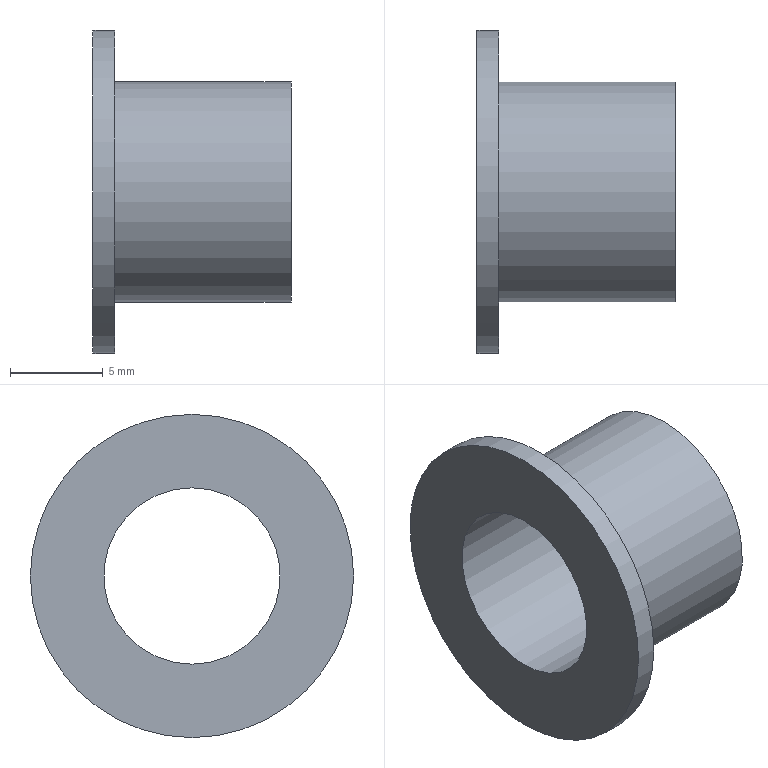Part | NX | features Igus GFI bushings(0.375 x 0.500) 2 | 1 solid | 6 faces | box 10.7 x 17.45 x 17.45 mm | volume 578.207 mm3 | plane 3 | cylinder 3 | commonest cylinder face diameters 9.525 x1 11.906 x1 17.45 x1
STEP:
#1=CARTESIAN_POINT('',(0.,0.,4.763));
#2=VERTEX_POINT('',#1);
#3=CARTESIAN_POINT('',(0.,0.,0.));
#4=DIRECTION('',(-1.,0.,0.));
#5=DIRECTION('',(0.,0.,1.));
#6=AXIS2_PLACEMENT_3D('',#3,#4,#5);
#7=CIRCLE('',#6,4.763);
#8=EDGE_CURVE('',#2,#2,#7,.T.);
#9=ORIENTED_EDGE('',*,*,#8,.F.);
#10=EDGE_LOOP('',(#9));
#11=FACE_BOUND('',#10,.T.);
#12=CARTESIAN_POINT('',(0.,0.,8.725));
#13=VERTEX_POINT('',#12);
#14=CARTESIAN_POINT('',(0.,0.,0.));
#15=DIRECTION('',(-1.,0.,0.));
#16=DIRECTION('',(0.,0.,1.));
#17=AXIS2_PLACEMENT_3D('',#14,#15,#16);
#18=CIRCLE('',#17,8.725);
#19=EDGE_CURVE('',#13,#13,#18,.T.);
#20=ORIENTED_EDGE('',*,*,#19,.T.);
#21=EDGE_LOOP('',(#20));
#22=FACE_BOUND('',#21,.T.);
#23=CARTESIAN_POINT('',(0.,4.763,0.));
#24=DIRECTION('',(1.,0.,0.));
#25=DIRECTION('',(0.,0.,-1.));
#26=AXIS2_PLACEMENT_3D('',#23,#24,#25);
#27=PLANE('',#26);
#28=ADVANCED_FACE('',(#11,#22),#27,.F.);
#29=CARTESIAN_POINT('',(10.7,0.,4.763));
#30=VERTEX_POINT('',#29);
#31=CARTESIAN_POINT('',(10.7,0.,0.));
#32=DIRECTION('',(-1.,0.,0.));
#33=DIRECTION('',(0.,0.,1.));
#34=AXIS2_PLACEMENT_3D('',#31,#32,#33);
#35=CIRCLE('',#34,4.763);
#36=EDGE_CURVE('',#30,#30,#35,.T.);
#37=ORIENTED_EDGE('',*,*,#36,.F.);
#38=EDGE_LOOP('',(#37));
#39=FACE_BOUND('',#38,.T.);
#40=ORIENTED_EDGE('',*,*,#8,.T.);
#41=EDGE_LOOP('',(#40));
#42=FACE_BOUND('',#41,.T.);
#43=CARTESIAN_POINT('',(0.,0.,0.));
#44=DIRECTION('',(-1.,0.,0.));
#45=DIRECTION('',(0.,0.,1.));
#46=AXIS2_PLACEMENT_3D('',#43,#44,#45);
#47=CYLINDRICAL_SURFACE('',#46,4.763);
#48=ADVANCED_FACE('',(#39,#42),#47,.F.);
#49=CARTESIAN_POINT('',(10.7,0.,5.953));
#50=VERTEX_POINT('',#49);
#51=CARTESIAN_POINT('',(10.7,0.,0.));
#52=DIRECTION('',(-1.,0.,0.));
#53=DIRECTION('',(0.,0.,1.));
#54=AXIS2_PLACEMENT_3D('',#51,#52,#53);
#55=CIRCLE('',#54,5.953);
#56=EDGE_CURVE('',#50,#50,#55,.T.);
#57=ORIENTED_EDGE('',*,*,#56,.F.);
#58=EDGE_LOOP('',(#57));
#59=FACE_BOUND('',#58,.T.);
#60=ORIENTED_EDGE('',*,*,#36,.T.);
#61=EDGE_LOOP('',(#60));
#62=FACE_BOUND('',#61,.T.);
#63=CARTESIAN_POINT('',(10.7,4.763,0.));
#64=DIRECTION('',(-1.,0.,0.));
#65=DIRECTION('',(0.,0.,1.));
#66=AXIS2_PLACEMENT_3D('',#63,#64,#65);
#67=PLANE('',#66);
#68=ADVANCED_FACE('',(#59,#62),#67,.F.);
#69=CARTESIAN_POINT('',(1.168,0.,5.953));
#70=VERTEX_POINT('',#69);
#71=CARTESIAN_POINT('',(1.168,0.,0.));
#72=DIRECTION('',(-1.,0.,0.));
#73=DIRECTION('',(0.,0.,1.));
#74=AXIS2_PLACEMENT_3D('',#71,#72,#73);
#75=CIRCLE('',#74,5.953);
#76=EDGE_CURVE('',#70,#70,#75,.T.);
#77=ORIENTED_EDGE('',*,*,#76,.F.);
#78=EDGE_LOOP('',(#77));
#79=FACE_BOUND('',#78,.T.);
#80=ORIENTED_EDGE('',*,*,#56,.T.);
#81=EDGE_LOOP('',(#80));
#82=FACE_BOUND('',#81,.T.);
#83=CARTESIAN_POINT('',(0.,0.,0.));
#84=DIRECTION('',(-1.,0.,0.));
#85=DIRECTION('',(0.,0.,1.));
#86=AXIS2_PLACEMENT_3D('',#83,#84,#85);
#87=CYLINDRICAL_SURFACE('',#86,5.953);
#88=ADVANCED_FACE('',(#79,#82),#87,.T.);
#89=CARTESIAN_POINT('',(1.168,0.,8.725));
#90=VERTEX_POINT('',#89);
#91=CARTESIAN_POINT('',(1.168,0.,0.));
#92=DIRECTION('',(-1.,0.,0.));
#93=DIRECTION('',(0.,0.,1.));
#94=AXIS2_PLACEMENT_3D('',#91,#92,#93);
#95=CIRCLE('',#94,8.725);
#96=EDGE_CURVE('',#90,#90,#95,.T.);
#97=ORIENTED_EDGE('',*,*,#96,.F.);
#98=EDGE_LOOP('',(#97));
#99=FACE_BOUND('',#98,.T.);
#100=ORIENTED_EDGE('',*,*,#76,.T.);
#101=EDGE_LOOP('',(#100));
#102=FACE_BOUND('',#101,.T.);
#103=CARTESIAN_POINT('',(1.168,5.953,0.));
#104=DIRECTION('',(-1.,0.,0.));
#105=DIRECTION('',(0.,0.,1.));
#106=AXIS2_PLACEMENT_3D('',#103,#104,#105);
#107=PLANE('',#106);
#108=ADVANCED_FACE('',(#99,#102),#107,.F.);
#109=ORIENTED_EDGE('',*,*,#19,.F.);
#110=EDGE_LOOP('',(#109));
#111=FACE_BOUND('',#110,.T.);
#112=ORIENTED_EDGE('',*,*,#96,.T.);
#113=EDGE_LOOP('',(#112));
#114=FACE_BOUND('',#113,.T.);
#115=CARTESIAN_POINT('',(0.,0.,0.));
#116=DIRECTION('',(-1.,0.,0.));
#117=DIRECTION('',(0.,0.,1.));
#118=AXIS2_PLACEMENT_3D('',#115,#116,#117);
#119=CYLINDRICAL_SURFACE('',#118,8.725);
#120=ADVANCED_FACE('',(#111,#114),#119,.T.);
#121=CLOSED_SHELL('',(#28,#48,#68,#88,#108,#120));
#122=MANIFOLD_SOLID_BREP('',#121);
#123=(LENGTH_UNIT()NAMED_UNIT(*)SI_UNIT(.MILLI.,.METRE.));
#124=UNCERTAINTY_MEASURE_WITH_UNIT(LENGTH_MEASURE(0.00001),#123,'','');
#125=(NAMED_UNIT(*)PLANE_ANGLE_UNIT()SI_UNIT($,.RADIAN.));
#126=(NAMED_UNIT(*)SI_UNIT($,.STERADIAN.)SOLID_ANGLE_UNIT());
#127=(GEOMETRIC_REPRESENTATION_CONTEXT(3)GLOBAL_UNCERTAINTY_ASSIGNED_CONTEXT((#124))GLOBAL_UNIT_ASSIGNED_CONTEXT((#123,#125,#126))REPRESENTATION_CONTEXT('',''));
#128=ADVANCED_BREP_SHAPE_REPRESENTATION('',(#122),#127);